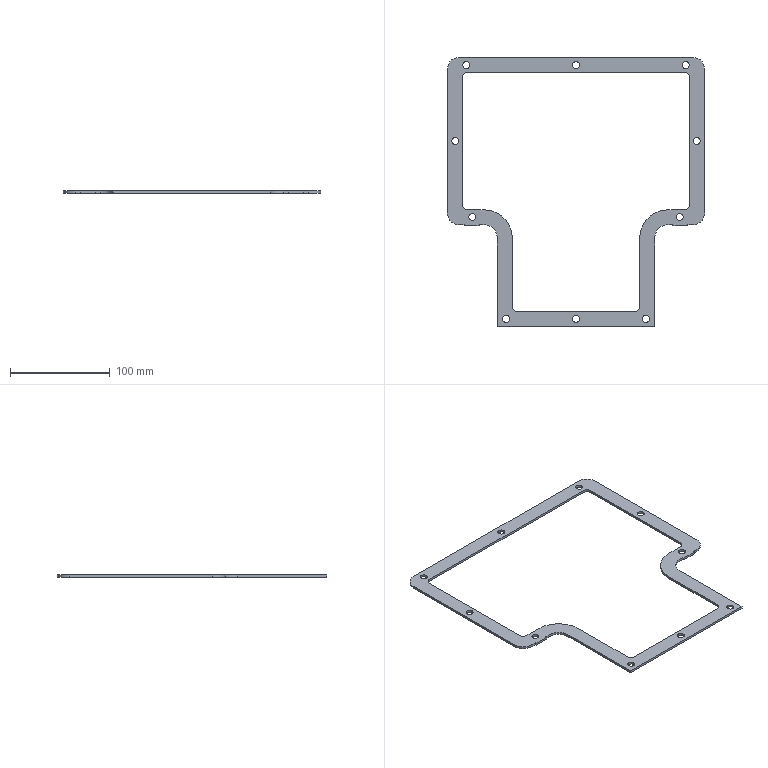Part | SolidWorks | features SMBaseFlange 2, FlatPattern 1, ICE 1, SheetMetal 1 | 1 solid | 60 faces | box 257.6 x 269.6 x 2.3 mm | volume 32681 mm3 | cylinder 34 | plane 26 | commonest cylinder face diameters 7 x20 10 x6 24 x4 26.4 x2 56.4 x2